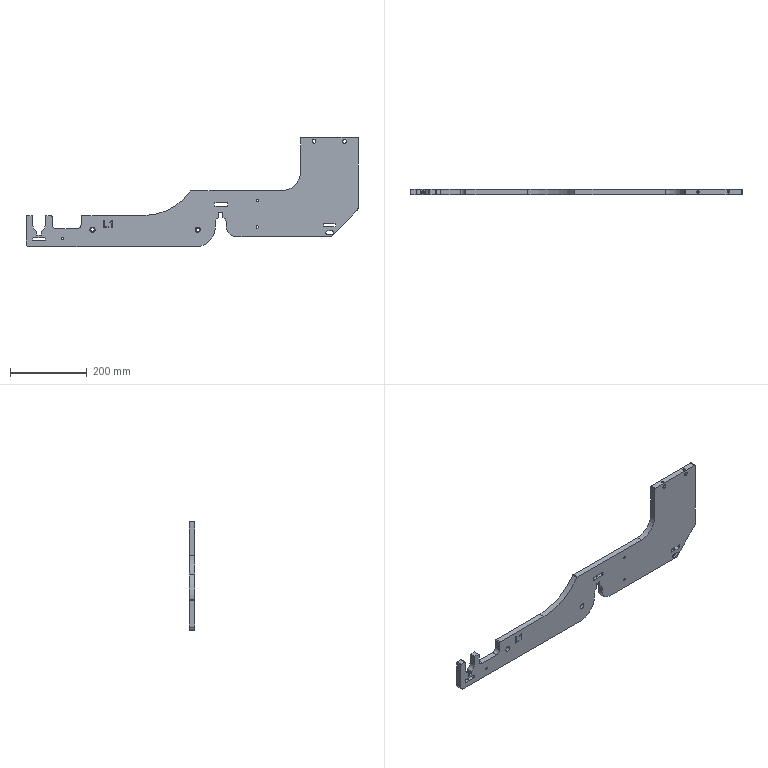Part | STEP file | Left | 1 solid | 120 faces | box 868 x 15 x 287 mm | volume 1544056 mm3 | plane 56 | cylinder 55 | cone 5 | other 4 | commonest cylinder face diameters 4 x16 6 x10 8 x5 5 x4 10 x4 9 x2